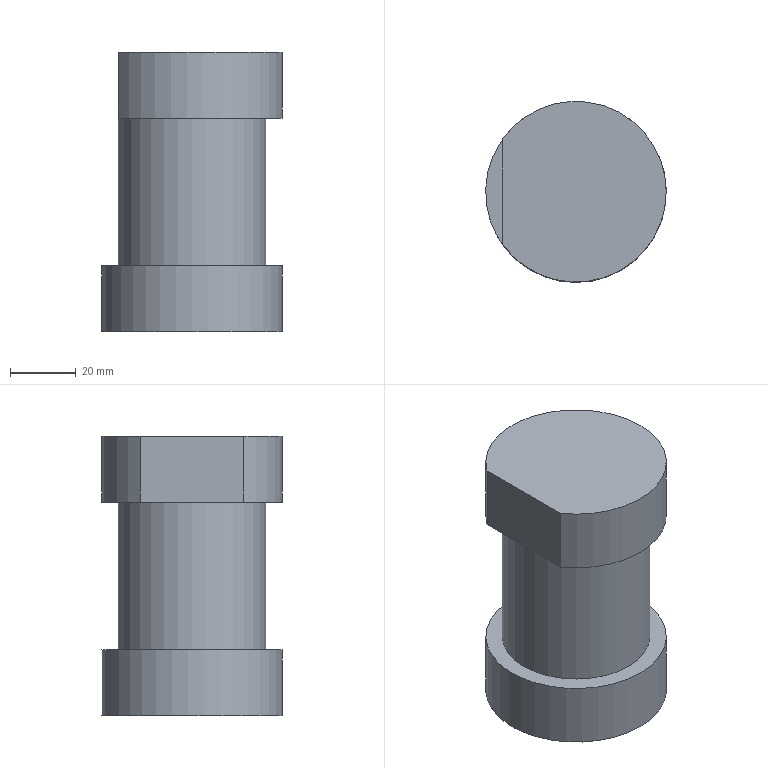Part | NX | features CSN24-TS162 2 | 1 solid | 11 faces | box 55 x 55 x 85 mm | volume 135381 mm3 | plane 5 | cylinder 4 | cone 2 | commonest cylinder face diameters 55 x2 22 x1 45 x1
STEP:
#1=CARTESIAN_POINT('',(887.5,230.,70.));
#2=VERTEX_POINT('',#1);
#3=CARTESIAN_POINT('',(887.5,245.811,70.));
#4=VERTEX_POINT('',#3);
#5=CARTESIAN_POINT('',(887.5,-270.,70.));
#6=DIRECTION('',(0.,1.,0.));
#7=VECTOR('',#6,1000.);
#8=LINE('',#5,#7);
#9=EDGE_CURVE('',#2,#4,#8,.T.);
#10=ORIENTED_EDGE('',*,*,#9,.T.);
#11=CARTESIAN_POINT('',(887.5,214.189,70.));
#12=VERTEX_POINT('',#11);
#13=CARTESIAN_POINT('',(910.,230.,70.));
#14=DIRECTION('',(0.,0.,1.));
#15=DIRECTION('',(0.,-1.,0.));
#16=AXIS2_PLACEMENT_3D('',#13,#14,#15);
#17=CIRCLE('',#16,27.5);
#18=EDGE_CURVE('',#12,#4,#17,.T.);
#19=ORIENTED_EDGE('',*,*,#18,.F.);
#20=CARTESIAN_POINT('',(887.5,-270.,70.));
#21=DIRECTION('',(0.,1.,0.));
#22=VECTOR('',#21,1000.);
#23=LINE('',#20,#22);
#24=EDGE_CURVE('',#12,#2,#23,.T.);
#25=ORIENTED_EDGE('',*,*,#24,.T.);
#26=CARTESIAN_POINT('',(910.,230.,70.));
#27=DIRECTION('',(0.,0.,1.));
#28=DIRECTION('',(0.,-1.,0.));
#29=AXIS2_PLACEMENT_3D('',#26,#27,#28);
#30=CIRCLE('',#29,22.5);
#31=EDGE_CURVE('',#2,#2,#30,.T.);
#32=ORIENTED_EDGE('',*,*,#31,.T.);
#33=EDGE_LOOP('',(#10,#19,#25,#32));
#34=FACE_BOUND('',#33,.T.);
#35=CARTESIAN_POINT('',(910.,252.5,70.));
#36=DIRECTION('',(0.,0.,1.));
#37=DIRECTION('',(0.,-1.,0.));
#38=AXIS2_PLACEMENT_3D('',#35,#36,#37);
#39=PLANE('',#38);
#40=ADVANCED_FACE('',(#34),#39,.F.);
#41=CARTESIAN_POINT('',(887.5,214.189,90.));
#42=VERTEX_POINT('',#41);
#43=CARTESIAN_POINT('',(887.5,214.189,5.));
#44=DIRECTION('',(0.,0.,1.));
#45=VECTOR('',#44,1000.);
#46=LINE('',#43,#45);
#47=EDGE_CURVE('',#12,#42,#46,.T.);
#48=ORIENTED_EDGE('',*,*,#47,.F.);
#49=ORIENTED_EDGE('',*,*,#18,.T.);
#50=CARTESIAN_POINT('',(887.5,245.811,90.));
#51=VERTEX_POINT('',#50);
#52=CARTESIAN_POINT('',(887.5,245.811,5.));
#53=DIRECTION('',(0.,0.,1.));
#54=VECTOR('',#53,1000.);
#55=LINE('',#52,#54);
#56=EDGE_CURVE('',#51,#4,#55,.F.);
#57=ORIENTED_EDGE('',*,*,#56,.F.);
#58=CARTESIAN_POINT('',(910.,230.,90.));
#59=DIRECTION('',(0.,0.,1.));
#60=DIRECTION('',(0.,-1.,0.));
#61=AXIS2_PLACEMENT_3D('',#58,#59,#60);
#62=CIRCLE('',#61,27.5);
#63=EDGE_CURVE('',#42,#51,#62,.T.);
#64=ORIENTED_EDGE('',*,*,#63,.F.);
#65=EDGE_LOOP('',(#48,#49,#57,#64));
#66=FACE_BOUND('',#65,.T.);
#67=CARTESIAN_POINT('',(910.,230.,5.));
#68=DIRECTION('',(0.,0.,1.));
#69=DIRECTION('',(0.,-1.,0.));
#70=AXIS2_PLACEMENT_3D('',#67,#68,#69);
#71=CYLINDRICAL_SURFACE('',#70,27.5);
#72=ADVANCED_FACE('',(#66),#71,.T.);
#73=CARTESIAN_POINT('',(887.5,257.5,90.));
#74=DIRECTION('',(0.,1.,0.));
#75=VECTOR('',#74,1000.);
#76=LINE('',#73,#75);
#77=EDGE_CURVE('',#42,#51,#76,.T.);
#78=ORIENTED_EDGE('',*,*,#77,.F.);
#79=ORIENTED_EDGE('',*,*,#63,.T.);
#80=EDGE_LOOP('',(#78,#79));
#81=FACE_BOUND('',#80,.T.);
#82=CARTESIAN_POINT('',(910.,257.5,90.));
#83=DIRECTION('',(0.,0.,-1.));
#84=DIRECTION('',(0.,1.,0.));
#85=AXIS2_PLACEMENT_3D('',#82,#83,#84);
#86=PLANE('',#85);
#87=ADVANCED_FACE('',(#81),#86,.F.);
#88=CARTESIAN_POINT('',(910.,202.5,5.));
#89=VERTEX_POINT('',#88);
#90=CARTESIAN_POINT('',(910.,230.,5.));
#91=DIRECTION('',(0.,0.,1.));
#92=DIRECTION('',(0.,-1.,0.));
#93=AXIS2_PLACEMENT_3D('',#90,#91,#92);
#94=CIRCLE('',#93,27.5);
#95=EDGE_CURVE('',#89,#89,#94,.T.);
#96=ORIENTED_EDGE('',*,*,#95,.F.);
#97=EDGE_LOOP('',(#96));
#98=FACE_BOUND('',#97,.T.);
#99=CARTESIAN_POINT('',(910.,207.5,5.));
#100=VERTEX_POINT('',#99);
#101=CARTESIAN_POINT('',(910.,230.,5.));
#102=DIRECTION('',(0.,0.,1.));
#103=DIRECTION('',(0.,-1.,0.));
#104=AXIS2_PLACEMENT_3D('',#101,#102,#103);
#105=CIRCLE('',#104,22.5);
#106=EDGE_CURVE('',#100,#100,#105,.T.);
#107=ORIENTED_EDGE('',*,*,#106,.T.);
#108=EDGE_LOOP('',(#107));
#109=FACE_BOUND('',#108,.T.);
#110=CARTESIAN_POINT('',(910.,252.5,5.));
#111=DIRECTION('',(0.,0.,1.));
#112=DIRECTION('',(0.,-1.,0.));
#113=AXIS2_PLACEMENT_3D('',#110,#111,#112);
#114=PLANE('',#113);
#115=ADVANCED_FACE('',(#98,#109),#114,.F.);
#116=CARTESIAN_POINT('',(910.,202.5,25.));
#117=VERTEX_POINT('',#116);
#118=CARTESIAN_POINT('',(910.,230.,25.));
#119=DIRECTION('',(0.,0.,1.));
#120=DIRECTION('',(0.,-1.,0.));
#121=AXIS2_PLACEMENT_3D('',#118,#119,#120);
#122=CIRCLE('',#121,27.5);
#123=EDGE_CURVE('',#117,#117,#122,.T.);
#124=ORIENTED_EDGE('',*,*,#123,.F.);
#125=EDGE_LOOP('',(#124));
#126=FACE_BOUND('',#125,.T.);
#127=ORIENTED_EDGE('',*,*,#95,.T.);
#128=EDGE_LOOP('',(#127));
#129=FACE_BOUND('',#128,.T.);
#130=CARTESIAN_POINT('',(910.,230.,5.));
#131=DIRECTION('',(0.,0.,1.));
#132=DIRECTION('',(0.,-1.,0.));
#133=AXIS2_PLACEMENT_3D('',#130,#131,#132);
#134=CYLINDRICAL_SURFACE('',#133,27.5);
#135=ADVANCED_FACE('',(#126,#129),#134,.T.);
#136=CARTESIAN_POINT('',(910.,207.5,25.));
#137=VERTEX_POINT('',#136);
#138=CARTESIAN_POINT('',(910.,230.,25.));
#139=DIRECTION('',(0.,0.,1.));
#140=DIRECTION('',(0.,-1.,0.));
#141=AXIS2_PLACEMENT_3D('',#138,#139,#140);
#142=CIRCLE('',#141,22.5);
#143=EDGE_CURVE('',#137,#137,#142,.T.);
#144=ORIENTED_EDGE('',*,*,#143,.F.);
#145=EDGE_LOOP('',(#144));
#146=FACE_BOUND('',#145,.T.);
#147=ORIENTED_EDGE('',*,*,#123,.T.);
#148=EDGE_LOOP('',(#147));
#149=FACE_BOUND('',#148,.T.);
#150=CARTESIAN_POINT('',(910.,257.5,25.));
#151=DIRECTION('',(0.,0.,-1.));
#152=DIRECTION('',(0.,1.,0.));
#153=AXIS2_PLACEMENT_3D('',#150,#151,#152);
#154=PLANE('',#153);
#155=ADVANCED_FACE('',(#146,#149),#154,.F.);
#156=ORIENTED_EDGE('',*,*,#31,.F.);
#157=EDGE_LOOP('',(#156));
#158=FACE_BOUND('',#157,.T.);
#159=ORIENTED_EDGE('',*,*,#143,.T.);
#160=EDGE_LOOP('',(#159));
#161=FACE_BOUND('',#160,.T.);
#162=CARTESIAN_POINT('',(910.,230.,5.));
#163=DIRECTION('',(0.,0.,1.));
#164=DIRECTION('',(0.,-1.,0.));
#165=AXIS2_PLACEMENT_3D('',#162,#163,#164);
#166=CYLINDRICAL_SURFACE('',#165,22.5);
#167=ADVANCED_FACE('',(#158,#161),#166,.T.);
#168=CARTESIAN_POINT('',(910.,219.,70.));
#169=VERTEX_POINT('',#168);
#170=CARTESIAN_POINT('',(910.,230.,70.));
#171=DIRECTION('',(0.,0.,1.));
#172=DIRECTION('',(0.,-1.,0.));
#173=AXIS2_PLACEMENT_3D('',#170,#171,#172);
#174=CIRCLE('',#173,11.);
#175=EDGE_CURVE('',#169,#169,#174,.T.);
#176=ORIENTED_EDGE('',*,*,#175,.F.);
#177=EDGE_LOOP('',(#176));
#178=FACE_BOUND('',#177,.T.);
#179=CARTESIAN_POINT('',(910.,230.,76.351));
#180=VERTEX_POINT('',#179);
#181=VERTEX_LOOP('',#180);
#182=FACE_BOUND('',#181,.T.);
#183=CARTESIAN_POINT('',(910.,230.,76.351));
#184=DIRECTION('',(0.,0.,-1.));
#185=DIRECTION('',(0.,1.,0.));
#186=AXIS2_PLACEMENT_3D('',#183,#184,#185);
#187=CONICAL_SURFACE('',#186,0.,1.047);
#188=ADVANCED_FACE('',(#178,#182),#187,.F.);
#189=CARTESIAN_POINT('',(910.,219.,11.64));
#190=VERTEX_POINT('',#189);
#191=CARTESIAN_POINT('',(910.,230.,11.64));
#192=DIRECTION('',(0.,0.,1.));
#193=DIRECTION('',(0.,-1.,0.));
#194=AXIS2_PLACEMENT_3D('',#191,#192,#193);
#195=CIRCLE('',#194,11.);
#196=EDGE_CURVE('',#190,#190,#195,.T.);
#197=ORIENTED_EDGE('',*,*,#196,.F.);
#198=EDGE_LOOP('',(#197));
#199=FACE_BOUND('',#198,.T.);
#200=ORIENTED_EDGE('',*,*,#175,.T.);
#201=EDGE_LOOP('',(#200));
#202=FACE_BOUND('',#201,.T.);
#203=CARTESIAN_POINT('',(910.,230.,5.));
#204=DIRECTION('',(0.,0.,1.));
#205=DIRECTION('',(0.,-1.,0.));
#206=AXIS2_PLACEMENT_3D('',#203,#204,#205);
#207=CYLINDRICAL_SURFACE('',#206,11.);
#208=ADVANCED_FACE('',(#199,#202),#207,.F.);
#209=ORIENTED_EDGE('',*,*,#106,.F.);
#210=EDGE_LOOP('',(#209));
#211=FACE_BOUND('',#210,.T.);
#212=ORIENTED_EDGE('',*,*,#196,.T.);
#213=EDGE_LOOP('',(#212));
#214=FACE_BOUND('',#213,.T.);
#215=CARTESIAN_POINT('',(910.,230.,11.64));
#216=DIRECTION('',(0.,0.,-1.));
#217=DIRECTION('',(0.,1.,0.));
#218=AXIS2_PLACEMENT_3D('',#215,#216,#217);
#219=CONICAL_SURFACE('',#218,11.,1.047);
#220=ADVANCED_FACE('',(#211,#214),#219,.F.);
#221=ORIENTED_EDGE('',*,*,#47,.T.);
#222=ORIENTED_EDGE('',*,*,#77,.T.);
#223=ORIENTED_EDGE('',*,*,#56,.T.);
#224=ORIENTED_EDGE('',*,*,#9,.F.);
#225=ORIENTED_EDGE('',*,*,#24,.F.);
#226=EDGE_LOOP('',(#221,#222,#223,#224,#225));
#227=FACE_BOUND('',#226,.T.);
#228=CARTESIAN_POINT('',(887.5,-270.,170.));
#229=DIRECTION('',(-1.,0.,0.));
#230=DIRECTION('',(0.,1.,0.));
#231=AXIS2_PLACEMENT_3D('',#228,#229,#230);
#232=PLANE('',#231);
#233=ADVANCED_FACE('',(#227),#232,.T.);
#234=CLOSED_SHELL('',(#40,#72,#87,#115,#135,#155,#167,#188,#208,#220,#233));
#235=MANIFOLD_SOLID_BREP('',#234);
#236=(LENGTH_UNIT()NAMED_UNIT(*)SI_UNIT(.MILLI.,.METRE.));
#237=UNCERTAINTY_MEASURE_WITH_UNIT(LENGTH_MEASURE(0.00001),#236,'','');
#238=(NAMED_UNIT(*)PLANE_ANGLE_UNIT()SI_UNIT($,.RADIAN.));
#239=(NAMED_UNIT(*)SI_UNIT($,.STERADIAN.)SOLID_ANGLE_UNIT());
#240=(GEOMETRIC_REPRESENTATION_CONTEXT(3)GLOBAL_UNCERTAINTY_ASSIGNED_CONTEXT((#237))GLOBAL_UNIT_ASSIGNED_CONTEXT((#236,#238,#239))REPRESENTATION_CONTEXT('',''));
#241=ADVANCED_BREP_SHAPE_REPRESENTATION('',(#235),#240);